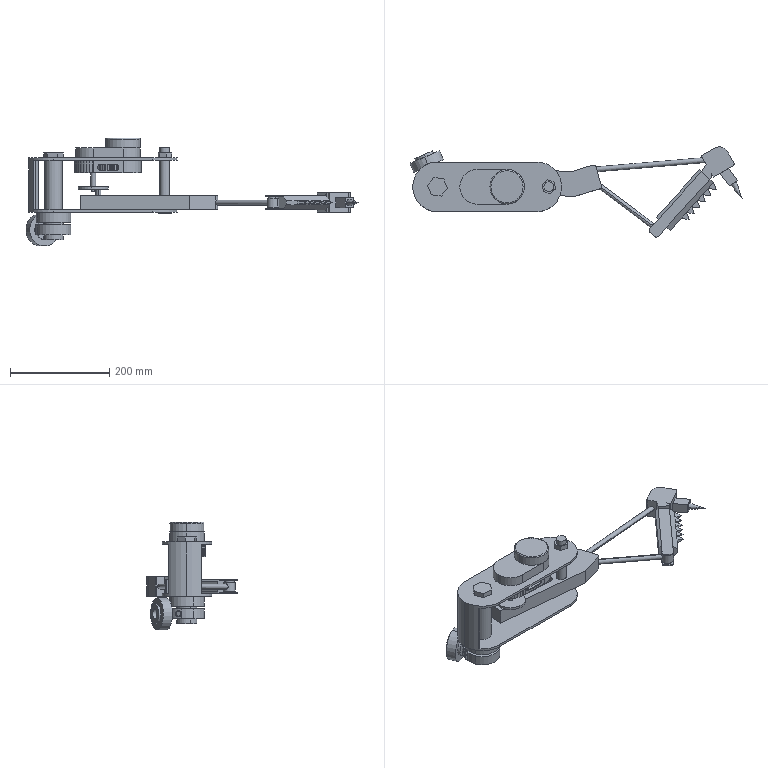Part | SolidWorks | 17 solids | 582 faces | box 668.994 x 181.738 x 217.5 mm | volume 1662687 mm3 | cylinder 398 | plane 176 | torus 6 | cone 2 | commonest cylinder face diameters 20 x97 28 x74 10 x36 64.998 x35 74 x35 44.998 x25